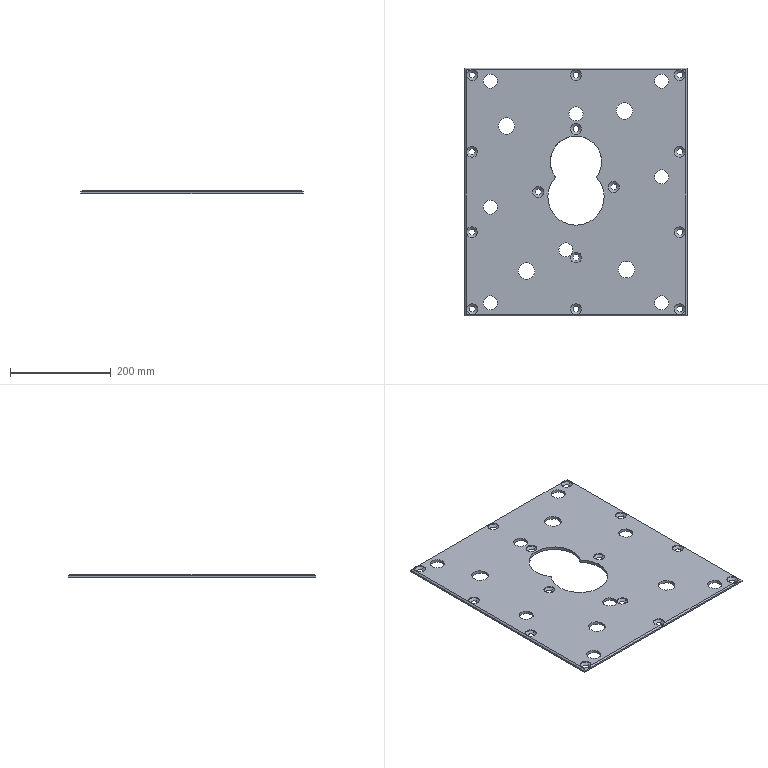Part | Creo | 1 solid | 92 faces | box 441 x 491 x 6 mm | volume 1122196 mm3 | cylinder 54 | cone 28 | plane 10 | commonest cylinder face diameters 21.5 x28 28 x16 33 x8 102 x1 112 x1